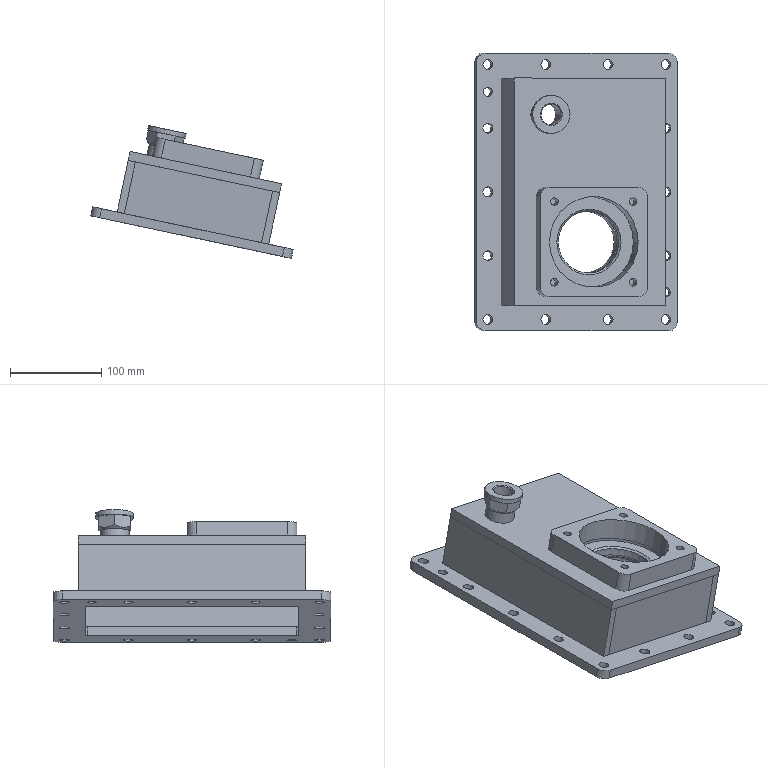Part | STEP file | HL4GZ-1.862.059 (gearbox housing) | 10 solids | 121 faces | box 222.162 x 305 x 145.748 mm | volume 1290088 mm3 | plane 69 | cylinder 48 | cone 4 | commonest cylinder face diameters 11 x14 20 x9 4 x4 8.376 x4 10 x2 68 x2